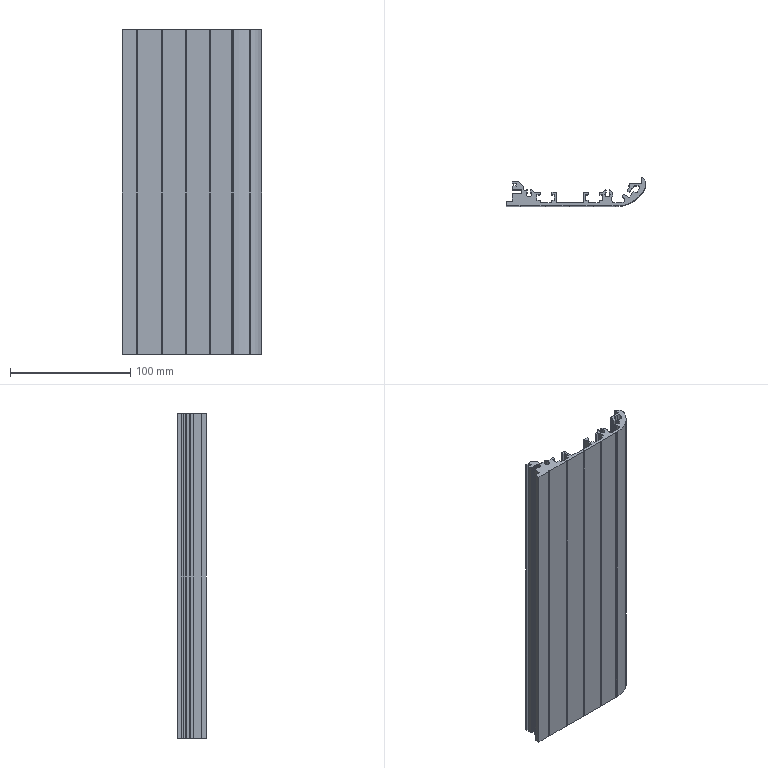Part | SolidWorks | features BaseBody 1 | 1 solid | 184 faces | box 116.267 x 23.727 x 270 mm | volume 211273 mm3 | plane 127 | cylinder 57 | commonest cylinder face diameters 1 x31 4.2 x6 2 x4 8.7 x4 2.4 x2 3 x2